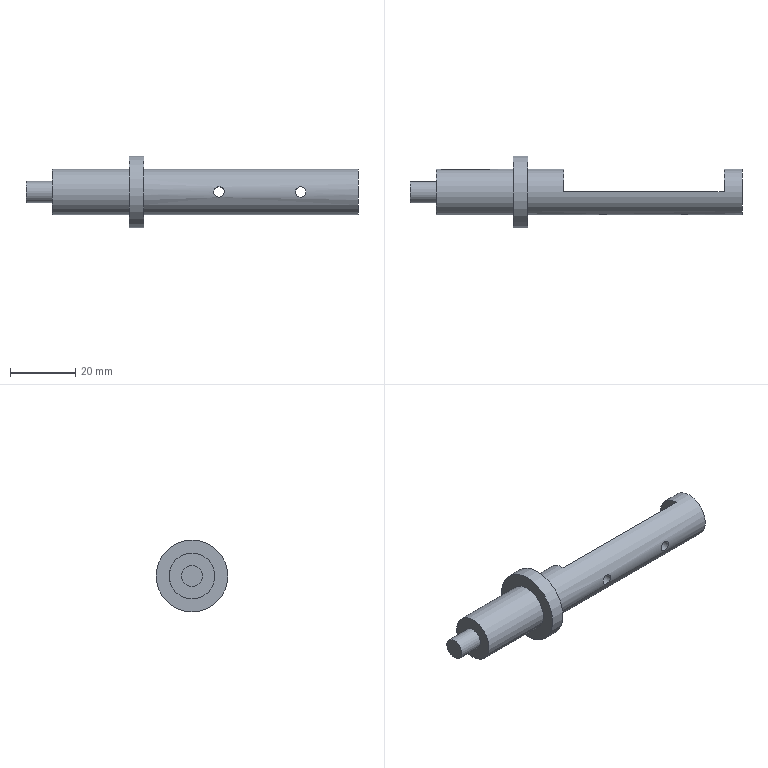Part | NX | features DATUM_CSYS 5, SKETCH 4, EXTRUDE 3, SWP104 1 | 1 solid | 17 faces | box 101.5 x 22 x 22 mm | volume 11635 mm3 | plane 10 | cylinder 7 | commonest cylinder face diameters 3.2 x2 14 x2 6.5 x1 16 x1 22 x1
STEP:
#1=CARTESIAN_POINT('',(36.,0.,-7.));
#2=VERTEX_POINT('',#1);
#3=CARTESIAN_POINT('',(36.,0.,0.));
#4=DIRECTION('',(1.,0.,0.));
#5=DIRECTION('',(0.,0.,-1.));
#6=AXIS2_PLACEMENT_3D('',#3,#4,#5);
#7=CIRCLE('',#6,7.);
#8=EDGE_CURVE('',#2,#2,#7,.T.);
#9=ORIENTED_EDGE('',*,*,#8,.T.);
#10=EDGE_LOOP('',(#9));
#11=FACE_BOUND('',#10,.T.);
#12=CARTESIAN_POINT('',(101.5,0.,-7.));
#13=VERTEX_POINT('',#12);
#14=CARTESIAN_POINT('',(101.5,0.,0.));
#15=DIRECTION('',(1.,0.,0.));
#16=DIRECTION('',(0.,0.,-1.));
#17=AXIS2_PLACEMENT_3D('',#14,#15,#16);
#18=CIRCLE('',#17,7.);
#19=EDGE_CURVE('',#13,#13,#18,.T.);
#20=ORIENTED_EDGE('',*,*,#19,.F.);
#21=EDGE_LOOP('',(#20));
#22=FACE_BOUND('',#21,.T.);
#23=CARTESIAN_POINT('',(47.,0.,-7.));
#24=VERTEX_POINT('',#23);
#25=CARTESIAN_POINT('',(47.,0.,7.));
#26=VERTEX_POINT('',#25);
#27=CARTESIAN_POINT('',(47.,0.,0.));
#28=DIRECTION('',(1.,0.,0.));
#29=DIRECTION('',(0.,0.,-1.));
#30=AXIS2_PLACEMENT_3D('',#27,#28,#29);
#31=CIRCLE('',#30,7.);
#32=EDGE_CURVE('',#24,#26,#31,.T.);
#33=ORIENTED_EDGE('',*,*,#32,.F.);
#34=CARTESIAN_POINT('',(96.,0.,-7.));
#35=VERTEX_POINT('',#34);
#36=CARTESIAN_POINT('',(0.,0.,-7.));
#37=DIRECTION('',(1.,0.,0.));
#38=VECTOR('',#37,1000.);
#39=LINE('',#36,#38);
#40=EDGE_CURVE('',#35,#24,#39,.F.);
#41=ORIENTED_EDGE('',*,*,#40,.F.);
#42=CARTESIAN_POINT('',(96.,0.,7.));
#43=VERTEX_POINT('',#42);
#44=CARTESIAN_POINT('',(96.,0.,0.));
#45=DIRECTION('',(-1.,0.,0.));
#46=DIRECTION('',(0.,0.,1.));
#47=AXIS2_PLACEMENT_3D('',#44,#45,#46);
#48=CIRCLE('',#47,7.);
#49=EDGE_CURVE('',#43,#35,#48,.T.);
#50=ORIENTED_EDGE('',*,*,#49,.F.);
#51=CARTESIAN_POINT('',(0.,0.,7.));
#52=DIRECTION('',(1.,0.,0.));
#53=VECTOR('',#52,1000.);
#54=LINE('',#51,#53);
#55=EDGE_CURVE('',#26,#43,#54,.T.);
#56=ORIENTED_EDGE('',*,*,#55,.F.);
#57=EDGE_LOOP('',(#33,#41,#50,#56));
#58=FACE_BOUND('',#57,.T.);
#59=CARTESIAN_POINT('',(60.6,-7.,0.));
#60=VERTEX_POINT('',#59);
#61=CARTESIAN_POINT('',(60.253,-6.908,-1.255));
#62=CARTESIAN_POINT('',(60.774,-7.046,0.0002562));
#63=CARTESIAN_POINT('',(60.253,-6.909,1.254));
#64=CARTESIAN_POINT('',(59.002,-6.768,1.773));
#65=CARTESIAN_POINT('',(57.746,-6.909,1.254));
#66=CARTESIAN_POINT('',(57.227,-7.046,0.0006779));
#67=CARTESIAN_POINT('',(57.745,-6.909,-1.253));
#68=CARTESIAN_POINT('',(58.999,-6.768,-1.773));
#69=CARTESIAN_POINT('',(60.253,-6.908,-1.255));
#70=CARTESIAN_POINT('',(60.774,-7.046,0.0002562));
#71=CARTESIAN_POINT('',(60.253,-6.909,1.254));
#72=B_SPLINE_CURVE_WITH_KNOTS('',3,(#61,#62,#63,#64,#65,#66,#67,#68,#69,#70,#71),.UNSPECIFIED.,.T.,.F.,(1,1,1,1,1,1,1,1,1,1,1,1,1,1,1),(-0.003764,-0.002509,-0.001255,0.,0.001255,0.002509,0.003764,0.005018,0.006273,0.007527,0.008782,0.01004,0.01129,0.01255,0.0138),.UNSPECIFIED.);
#73=EDGE_CURVE('',#60,#60,#72,.T.);
#74=ORIENTED_EDGE('',*,*,#73,.F.);
#75=EDGE_LOOP('',(#74));
#76=FACE_BOUND('',#75,.T.);
#77=CARTESIAN_POINT('',(85.6,-7.,0.));
#78=VERTEX_POINT('',#77);
#79=CARTESIAN_POINT('',(85.253,-6.908,-1.255));
#80=CARTESIAN_POINT('',(85.774,-7.046,0.0002562));
#81=CARTESIAN_POINT('',(85.253,-6.909,1.254));
#82=CARTESIAN_POINT('',(84.002,-6.768,1.773));
#83=CARTESIAN_POINT('',(82.746,-6.909,1.254));
#84=CARTESIAN_POINT('',(82.227,-7.046,0.0006779));
#85=CARTESIAN_POINT('',(82.745,-6.909,-1.253));
#86=CARTESIAN_POINT('',(83.999,-6.768,-1.773));
#87=CARTESIAN_POINT('',(85.253,-6.908,-1.255));
#88=CARTESIAN_POINT('',(85.774,-7.046,0.0002562));
#89=CARTESIAN_POINT('',(85.253,-6.909,1.254));
#90=B_SPLINE_CURVE_WITH_KNOTS('',3,(#79,#80,#81,#82,#83,#84,#85,#86,#87,#88,#89),.UNSPECIFIED.,.T.,.F.,(1,1,1,1,1,1,1,1,1,1,1,1,1,1,1),(-0.003764,-0.002509,-0.001255,0.,0.001255,0.002509,0.003764,0.005018,0.006273,0.007527,0.008782,0.01004,0.01129,0.01255,0.0138),.UNSPECIFIED.);
#91=EDGE_CURVE('',#78,#78,#90,.T.);
#92=ORIENTED_EDGE('',*,*,#91,.F.);
#93=EDGE_LOOP('',(#92));
#94=FACE_BOUND('',#93,.T.);
#95=CARTESIAN_POINT('',(0.,0.,0.));
#96=DIRECTION('',(1.,0.,0.));
#97=DIRECTION('',(0.,0.,-1.));
#98=AXIS2_PLACEMENT_3D('',#95,#96,#97);
#99=CYLINDRICAL_SURFACE('',#98,7.);
#100=ADVANCED_FACE('',(#11,#22,#58,#76,#94),#99,.T.);
#101=CARTESIAN_POINT('',(31.5,0.,-7.));
#102=VERTEX_POINT('',#101);
#103=CARTESIAN_POINT('',(31.5,0.,0.));
#104=DIRECTION('',(1.,0.,0.));
#105=DIRECTION('',(0.,0.,-1.));
#106=AXIS2_PLACEMENT_3D('',#103,#104,#105);
#107=CIRCLE('',#106,7.);
#108=EDGE_CURVE('',#102,#102,#107,.T.);
#109=ORIENTED_EDGE('',*,*,#108,.F.);
#110=EDGE_LOOP('',(#109));
#111=FACE_BOUND('',#110,.T.);
#112=CARTESIAN_POINT('',(8.,0.,-7.));
#113=VERTEX_POINT('',#112);
#114=CARTESIAN_POINT('',(8.,0.,0.));
#115=DIRECTION('',(1.,0.,0.));
#116=DIRECTION('',(0.,0.,-1.));
#117=AXIS2_PLACEMENT_3D('',#114,#115,#116);
#118=CIRCLE('',#117,7.);
#119=EDGE_CURVE('',#113,#113,#118,.T.);
#120=ORIENTED_EDGE('',*,*,#119,.T.);
#121=EDGE_LOOP('',(#120));
#122=FACE_BOUND('',#121,.T.);
#123=CARTESIAN_POINT('',(24.348,6.837,1.5));
#124=VERTEX_POINT('',#123);
#125=CARTESIAN_POINT('',(9.652,6.837,1.5));
#126=VERTEX_POINT('',#125);
#127=CARTESIAN_POINT('',(0.,6.837,1.5));
#128=DIRECTION('',(1.,0.,0.));
#129=VECTOR('',#128,1000.);
#130=LINE('',#127,#129);
#131=EDGE_CURVE('',#124,#126,#130,.F.);
#132=ORIENTED_EDGE('',*,*,#131,.T.);
#133=CARTESIAN_POINT('',(9.652,6.837,-1.5));
#134=VERTEX_POINT('',#133);
#135=CARTESIAN_POINT('',(9.652,6.837,-1.5));
#136=CARTESIAN_POINT('',(9.558,7.054,-0.5112));
#137=CARTESIAN_POINT('',(9.558,7.054,0.5113));
#138=CARTESIAN_POINT('',(9.652,6.837,1.5));
#139=B_SPLINE_CURVE_WITH_KNOTS('',3,(#135,#136,#137,#138),.UNSPECIFIED.,.F.,.F.,(4,4),(0.,0.003007),.UNSPECIFIED.);
#140=EDGE_CURVE('',#134,#126,#139,.T.);
#141=ORIENTED_EDGE('',*,*,#140,.F.);
#142=CARTESIAN_POINT('',(24.348,6.837,-1.5));
#143=VERTEX_POINT('',#142);
#144=CARTESIAN_POINT('',(0.,6.837,-1.5));
#145=DIRECTION('',(1.,0.,0.));
#146=VECTOR('',#145,1000.);
#147=LINE('',#144,#146);
#148=EDGE_CURVE('',#143,#134,#147,.F.);
#149=ORIENTED_EDGE('',*,*,#148,.F.);
#150=CARTESIAN_POINT('',(24.348,6.837,1.5));
#151=CARTESIAN_POINT('',(24.442,7.054,0.5112));
#152=CARTESIAN_POINT('',(24.442,7.054,-0.5113));
#153=CARTESIAN_POINT('',(24.348,6.837,-1.5));
#154=B_SPLINE_CURVE_WITH_KNOTS('',3,(#150,#151,#152,#153),.UNSPECIFIED.,.F.,.F.,(4,4),(0.,0.003007),.UNSPECIFIED.);
#155=EDGE_CURVE('',#124,#143,#154,.T.);
#156=ORIENTED_EDGE('',*,*,#155,.F.);
#157=EDGE_LOOP('',(#132,#141,#149,#156));
#158=FACE_BOUND('',#157,.T.);
#159=CARTESIAN_POINT('',(0.,0.,0.));
#160=DIRECTION('',(1.,0.,0.));
#161=DIRECTION('',(0.,0.,-1.));
#162=AXIS2_PLACEMENT_3D('',#159,#160,#161);
#163=CYLINDRICAL_SURFACE('',#162,7.);
#164=ADVANCED_FACE('',(#111,#122,#158),#163,.T.);
#165=CARTESIAN_POINT('',(0.,0.,-3.25));
#166=VERTEX_POINT('',#165);
#167=CARTESIAN_POINT('',(0.,0.,0.));
#168=DIRECTION('',(1.,0.,0.));
#169=DIRECTION('',(0.,0.,-1.));
#170=AXIS2_PLACEMENT_3D('',#167,#168,#169);
#171=CIRCLE('',#170,3.25);
#172=EDGE_CURVE('',#166,#166,#171,.T.);
#173=ORIENTED_EDGE('',*,*,#172,.F.);
#174=EDGE_LOOP('',(#173));
#175=FACE_BOUND('',#174,.T.);
#176=CARTESIAN_POINT('',(0.,0.,0.));
#177=DIRECTION('',(1.,0.,0.));
#178=DIRECTION('',(0.,0.,-1.));
#179=AXIS2_PLACEMENT_3D('',#176,#177,#178);
#180=PLANE('',#179);
#181=ADVANCED_FACE('',(#175),#180,.F.);
#182=CARTESIAN_POINT('',(8.,0.,-3.25));
#183=VERTEX_POINT('',#182);
#184=CARTESIAN_POINT('',(8.,0.,0.));
#185=DIRECTION('',(1.,0.,0.));
#186=DIRECTION('',(0.,0.,-1.));
#187=AXIS2_PLACEMENT_3D('',#184,#185,#186);
#188=CIRCLE('',#187,3.25);
#189=EDGE_CURVE('',#183,#183,#188,.T.);
#190=ORIENTED_EDGE('',*,*,#189,.F.);
#191=EDGE_LOOP('',(#190));
#192=FACE_BOUND('',#191,.T.);
#193=ORIENTED_EDGE('',*,*,#172,.T.);
#194=EDGE_LOOP('',(#193));
#195=FACE_BOUND('',#194,.T.);
#196=CARTESIAN_POINT('',(0.,0.,0.));
#197=DIRECTION('',(1.,0.,0.));
#198=DIRECTION('',(0.,0.,-1.));
#199=AXIS2_PLACEMENT_3D('',#196,#197,#198);
#200=CYLINDRICAL_SURFACE('',#199,3.25);
#201=ADVANCED_FACE('',(#192,#195),#200,.T.);
#202=ORIENTED_EDGE('',*,*,#119,.F.);
#203=EDGE_LOOP('',(#202));
#204=FACE_BOUND('',#203,.T.);
#205=ORIENTED_EDGE('',*,*,#189,.T.);
#206=EDGE_LOOP('',(#205));
#207=FACE_BOUND('',#206,.T.);
#208=CARTESIAN_POINT('',(8.,3.25,0.));
#209=DIRECTION('',(1.,0.,0.));
#210=DIRECTION('',(0.,0.,-1.));
#211=AXIS2_PLACEMENT_3D('',#208,#209,#210);
#212=PLANE('',#211);
#213=ADVANCED_FACE('',(#204,#207),#212,.F.);
#214=CARTESIAN_POINT('',(31.5,0.,-11.));
#215=VERTEX_POINT('',#214);
#216=CARTESIAN_POINT('',(31.5,0.,0.));
#217=DIRECTION('',(1.,0.,0.));
#218=DIRECTION('',(0.,0.,-1.));
#219=AXIS2_PLACEMENT_3D('',#216,#217,#218);
#220=CIRCLE('',#219,11.);
#221=EDGE_CURVE('',#215,#215,#220,.T.);
#222=ORIENTED_EDGE('',*,*,#221,.F.);
#223=EDGE_LOOP('',(#222));
#224=FACE_BOUND('',#223,.T.);
#225=ORIENTED_EDGE('',*,*,#108,.T.);
#226=EDGE_LOOP('',(#225));
#227=FACE_BOUND('',#226,.T.);
#228=CARTESIAN_POINT('',(31.5,7.,0.));
#229=DIRECTION('',(1.,0.,0.));
#230=DIRECTION('',(0.,0.,-1.));
#231=AXIS2_PLACEMENT_3D('',#228,#229,#230);
#232=PLANE('',#231);
#233=ADVANCED_FACE('',(#224,#227),#232,.F.);
#234=CARTESIAN_POINT('',(36.,0.,-11.));
#235=VERTEX_POINT('',#234);
#236=CARTESIAN_POINT('',(36.,0.,0.));
#237=DIRECTION('',(1.,0.,0.));
#238=DIRECTION('',(0.,0.,-1.));
#239=AXIS2_PLACEMENT_3D('',#236,#237,#238);
#240=CIRCLE('',#239,11.);
#241=EDGE_CURVE('',#235,#235,#240,.T.);
#242=ORIENTED_EDGE('',*,*,#241,.F.);
#243=EDGE_LOOP('',(#242));
#244=FACE_BOUND('',#243,.T.);
#245=ORIENTED_EDGE('',*,*,#221,.T.);
#246=EDGE_LOOP('',(#245));
#247=FACE_BOUND('',#246,.T.);
#248=CARTESIAN_POINT('',(0.,0.,0.));
#249=DIRECTION('',(1.,0.,0.));
#250=DIRECTION('',(0.,0.,-1.));
#251=AXIS2_PLACEMENT_3D('',#248,#249,#250);
#252=CYLINDRICAL_SURFACE('',#251,11.);
#253=ADVANCED_FACE('',(#244,#247),#252,.T.);
#254=ORIENTED_EDGE('',*,*,#8,.F.);
#255=EDGE_LOOP('',(#254));
#256=FACE_BOUND('',#255,.T.);
#257=ORIENTED_EDGE('',*,*,#241,.T.);
#258=EDGE_LOOP('',(#257));
#259=FACE_BOUND('',#258,.T.);
#260=CARTESIAN_POINT('',(36.,11.,0.));
#261=DIRECTION('',(-1.,0.,0.));
#262=DIRECTION('',(0.,0.,1.));
#263=AXIS2_PLACEMENT_3D('',#260,#261,#262);
#264=PLANE('',#263);
#265=ADVANCED_FACE('',(#256,#259),#264,.F.);
#266=ORIENTED_EDGE('',*,*,#19,.T.);
#267=EDGE_LOOP('',(#266));
#268=FACE_BOUND('',#267,.T.);
#269=CARTESIAN_POINT('',(101.5,7.,0.));
#270=DIRECTION('',(-1.,0.,0.));
#271=DIRECTION('',(0.,0.,1.));
#272=AXIS2_PLACEMENT_3D('',#269,#270,#271);
#273=PLANE('',#272);
#274=ADVANCED_FACE('',(#268),#273,.F.);
#275=ORIENTED_EDGE('',*,*,#32,.T.);
#276=CARTESIAN_POINT('',(47.,0.,16.5));
#277=DIRECTION('',(0.,0.,-1.));
#278=VECTOR('',#277,1000.);
#279=LINE('',#276,#278);
#280=EDGE_CURVE('',#24,#26,#279,.F.);
#281=ORIENTED_EDGE('',*,*,#280,.F.);
#282=EDGE_LOOP('',(#275,#281));
#283=FACE_BOUND('',#282,.T.);
#284=CARTESIAN_POINT('',(47.,10.,16.5));
#285=DIRECTION('',(1.,0.,0.));
#286=DIRECTION('',(0.,0.,-1.));
#287=AXIS2_PLACEMENT_3D('',#284,#285,#286);
#288=PLANE('',#287);
#289=ADVANCED_FACE('',(#283),#288,.T.);
#290=CARTESIAN_POINT('',(82.4,0.,0.));
#291=VERTEX_POINT('',#290);
#292=CARTESIAN_POINT('',(84.,0.,0.));
#293=DIRECTION('',(0.,1.,0.));
#294=DIRECTION('',(-1.,0.,0.));
#295=AXIS2_PLACEMENT_3D('',#292,#293,#294);
#296=CIRCLE('',#295,1.6);
#297=EDGE_CURVE('',#291,#291,#296,.F.);
#298=ORIENTED_EDGE('',*,*,#297,.T.);
#299=EDGE_LOOP('',(#298));
#300=FACE_BOUND('',#299,.T.);
#301=CARTESIAN_POINT('',(57.4,0.,0.));
#302=VERTEX_POINT('',#301);
#303=CARTESIAN_POINT('',(59.,0.,0.));
#304=DIRECTION('',(0.,1.,0.));
#305=DIRECTION('',(-1.,0.,0.));
#306=AXIS2_PLACEMENT_3D('',#303,#304,#305);
#307=CIRCLE('',#306,1.6);
#308=EDGE_CURVE('',#302,#302,#307,.F.);
#309=ORIENTED_EDGE('',*,*,#308,.T.);
#310=EDGE_LOOP('',(#309));
#311=FACE_BOUND('',#310,.T.);
#312=ORIENTED_EDGE('',*,*,#55,.T.);
#313=CARTESIAN_POINT('',(96.,0.,16.5));
#314=DIRECTION('',(0.,0.,-1.));
#315=VECTOR('',#314,1000.);
#316=LINE('',#313,#315);
#317=EDGE_CURVE('',#35,#43,#316,.F.);
#318=ORIENTED_EDGE('',*,*,#317,.F.);
#319=ORIENTED_EDGE('',*,*,#40,.T.);
#320=ORIENTED_EDGE('',*,*,#280,.T.);
#321=EDGE_LOOP('',(#312,#318,#319,#320));
#322=FACE_BOUND('',#321,.T.);
#323=CARTESIAN_POINT('',(47.,0.,16.5));
#324=DIRECTION('',(0.,1.,0.));
#325=DIRECTION('',(-1.,0.,0.));
#326=AXIS2_PLACEMENT_3D('',#323,#324,#325);
#327=PLANE('',#326);
#328=ADVANCED_FACE('',(#300,#311,#322),#327,.T.);
#329=ORIENTED_EDGE('',*,*,#49,.T.);
#330=ORIENTED_EDGE('',*,*,#317,.T.);
#331=EDGE_LOOP('',(#329,#330));
#332=FACE_BOUND('',#331,.T.);
#333=CARTESIAN_POINT('',(96.,0.,16.5));
#334=DIRECTION('',(-1.,0.,0.));
#335=DIRECTION('',(0.,0.,1.));
#336=AXIS2_PLACEMENT_3D('',#333,#334,#335);
#337=PLANE('',#336);
#338=ADVANCED_FACE('',(#332),#337,.T.);
#339=CARTESIAN_POINT('',(17.,10.,1.5));
#340=DIRECTION('',(0.,0.,1.));
#341=DIRECTION('',(1.,0.,0.));
#342=AXIS2_PLACEMENT_3D('',#339,#340,#341);
#343=CIRCLE('',#342,8.);
#344=EDGE_CURVE('',#124,#126,#343,.F.);
#345=ORIENTED_EDGE('',*,*,#344,.F.);
#346=ORIENTED_EDGE('',*,*,#155,.T.);
#347=CARTESIAN_POINT('',(17.,10.,-1.5));
#348=DIRECTION('',(0.,0.,1.));
#349=DIRECTION('',(1.,0.,0.));
#350=AXIS2_PLACEMENT_3D('',#347,#348,#349);
#351=CIRCLE('',#350,8.);
#352=EDGE_CURVE('',#143,#134,#351,.F.);
#353=ORIENTED_EDGE('',*,*,#352,.T.);
#354=ORIENTED_EDGE('',*,*,#140,.T.);
#355=EDGE_LOOP('',(#345,#346,#353,#354));
#356=FACE_BOUND('',#355,.T.);
#357=CARTESIAN_POINT('',(17.,10.,1.5));
#358=DIRECTION('',(0.,0.,-1.));
#359=DIRECTION('',(-1.,0.,0.));
#360=AXIS2_PLACEMENT_3D('',#357,#358,#359);
#361=CYLINDRICAL_SURFACE('',#360,8.);
#362=ADVANCED_FACE('',(#356),#361,.F.);
#363=ORIENTED_EDGE('',*,*,#344,.T.);
#364=ORIENTED_EDGE('',*,*,#131,.F.);
#365=EDGE_LOOP('',(#363,#364));
#366=FACE_BOUND('',#365,.T.);
#367=CARTESIAN_POINT('',(17.,10.,1.5));
#368=DIRECTION('',(0.,0.,1.));
#369=DIRECTION('',(1.,0.,0.));
#370=AXIS2_PLACEMENT_3D('',#367,#368,#369);
#371=PLANE('',#370);
#372=ADVANCED_FACE('',(#366),#371,.F.);
#373=ORIENTED_EDGE('',*,*,#148,.T.);
#374=ORIENTED_EDGE('',*,*,#352,.F.);
#375=EDGE_LOOP('',(#373,#374));
#376=FACE_BOUND('',#375,.T.);
#377=CARTESIAN_POINT('',(17.,10.,-1.5));
#378=DIRECTION('',(0.,0.,1.));
#379=DIRECTION('',(1.,0.,0.));
#380=AXIS2_PLACEMENT_3D('',#377,#378,#379);
#381=PLANE('',#380);
#382=ADVANCED_FACE('',(#376),#381,.T.);
#383=ORIENTED_EDGE('',*,*,#308,.F.);
#384=EDGE_LOOP('',(#383));
#385=FACE_BOUND('',#384,.T.);
#386=ORIENTED_EDGE('',*,*,#73,.T.);
#387=EDGE_LOOP('',(#386));
#388=FACE_BOUND('',#387,.T.);
#389=CARTESIAN_POINT('',(59.,16.5,0.));
#390=DIRECTION('',(0.,-1.,0.));
#391=DIRECTION('',(1.,0.,0.));
#392=AXIS2_PLACEMENT_3D('',#389,#390,#391);
#393=CYLINDRICAL_SURFACE('',#392,1.6);
#394=ADVANCED_FACE('',(#385,#388),#393,.F.);
#395=ORIENTED_EDGE('',*,*,#297,.F.);
#396=EDGE_LOOP('',(#395));
#397=FACE_BOUND('',#396,.T.);
#398=ORIENTED_EDGE('',*,*,#91,.T.);
#399=EDGE_LOOP('',(#398));
#400=FACE_BOUND('',#399,.T.);
#401=CARTESIAN_POINT('',(84.,16.5,0.));
#402=DIRECTION('',(0.,-1.,0.));
#403=DIRECTION('',(1.,0.,0.));
#404=AXIS2_PLACEMENT_3D('',#401,#402,#403);
#405=CYLINDRICAL_SURFACE('',#404,1.6);
#406=ADVANCED_FACE('',(#397,#400),#405,.F.);
#407=CLOSED_SHELL('',(#100,#164,#181,#201,#213,#233,#253,#265,#274,#289,#328,#338,#362,#372,#382,#394,#406));
#408=MANIFOLD_SOLID_BREP('',#407);
#409=(LENGTH_UNIT()NAMED_UNIT(*)SI_UNIT(.MILLI.,.METRE.));
#410=UNCERTAINTY_MEASURE_WITH_UNIT(LENGTH_MEASURE(0.0508),#409,'','');
#411=(NAMED_UNIT(*)PLANE_ANGLE_UNIT()SI_UNIT($,.RADIAN.));
#412=(NAMED_UNIT(*)SI_UNIT($,.STERADIAN.)SOLID_ANGLE_UNIT());
#413=(GEOMETRIC_REPRESENTATION_CONTEXT(3)GLOBAL_UNCERTAINTY_ASSIGNED_CONTEXT((#410))GLOBAL_UNIT_ASSIGNED_CONTEXT((#409,#411,#412))REPRESENTATION_CONTEXT('',''));
#414=ADVANCED_BREP_SHAPE_REPRESENTATION('',(#408),#413);